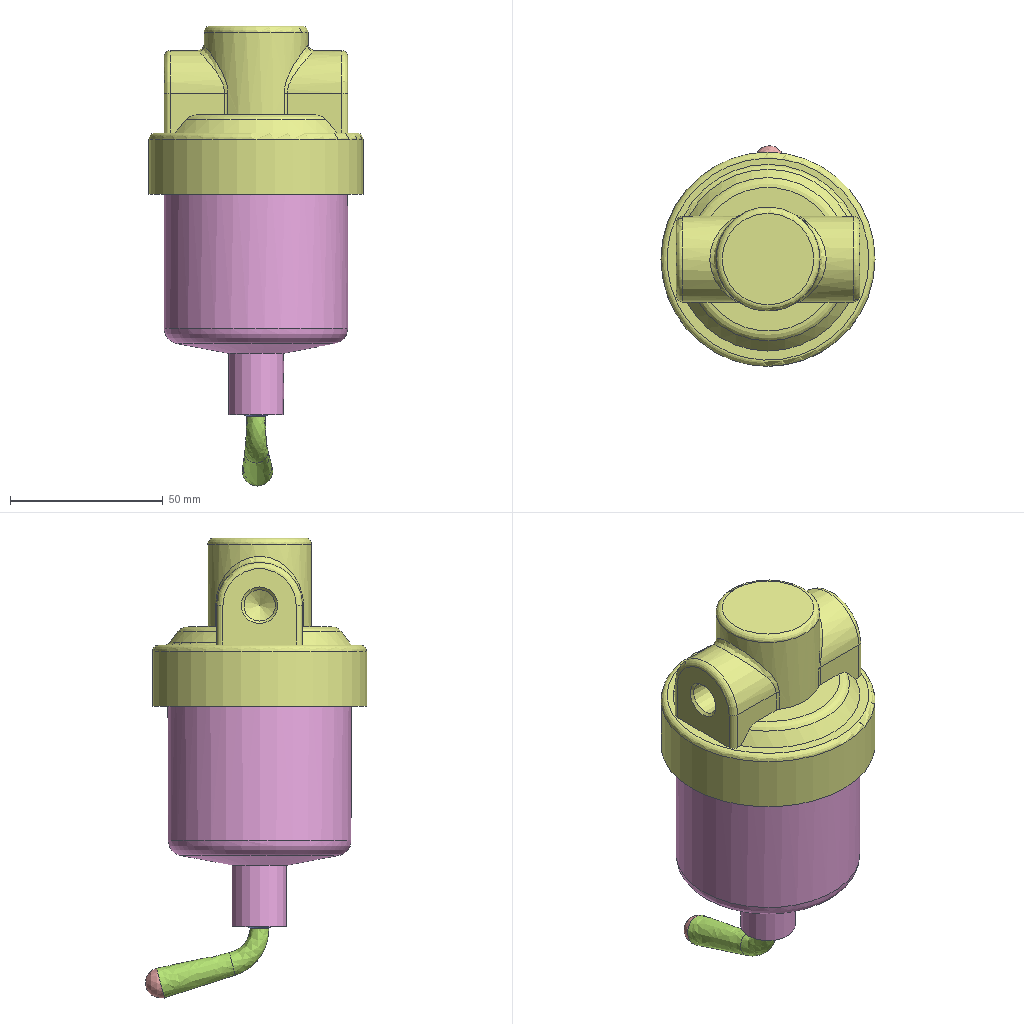Assembly | NX | 9 different items | 9 placed | box 70 x 72 x 150 mm
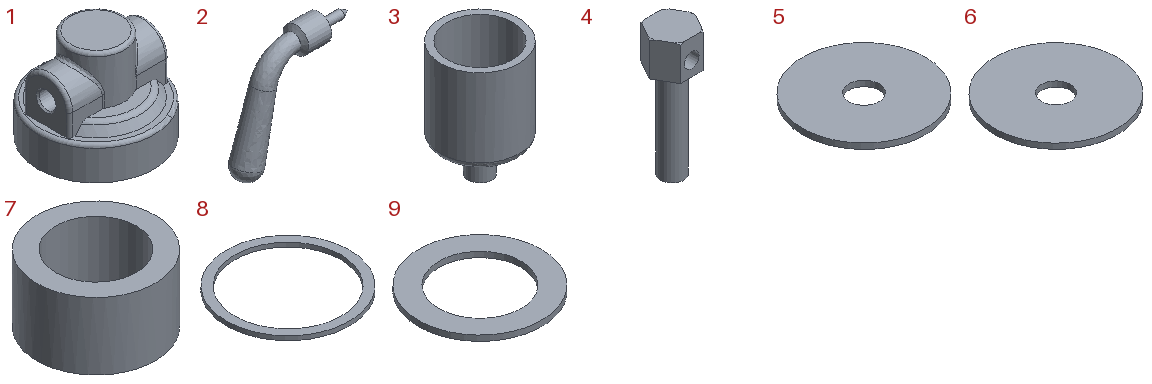Parts list (item | quantity | size | volume | features):
1 | x1 | 70 x 70 x 55 mm | 79994 mm3 | features CYLINDER 5, HOLE PACKAGE 5, SIMPLE HOLE 5, SYMBOLIC_THREAD 4, BLEND 3, DATUM_CSYS 2, BLOCK 1, SKETCH 1, SWP104 1
2 | x1 | 43.874 x 10 x 42.344 mm | 3412 mm3 | features SKETCH 4, DATUM_CSYS 3, DATUM_ON_PATH 2, SKIN 1, SPHERE 1, SWP104 1
3 | x1 | 60 x 60 x 88 mm | 68833 mm3 | features CYLINDER 3, BLEND 2, DATUM_CSYS 2, HOLE PACKAGE 2, SIMPLE HOLE 2, SYMBOLIC_THREAD 2, SKETCH 1, SWP104 1
4 | x1 | 18.475 x 16 x 52 mm | 4103 mm3 | features DATUM_CSYS 3, EXTRUDE 3, SKETCH 2, CHAMFER 1, CYLINDER 1, HOLE PACKAGE 1, SIMPLE HOLE 1, SYMBOLIC_THREAD 1
5 | x1 | 44 x 44 x 2 mm | 2851 mm3 | features CYLINDER 1, DATUM_CSYS 1, HOLE PACKAGE 1, SIMPLE HOLE 1
6 | x1 | 46 x 46 x 2 mm | 3134 mm3 | features CYLINDER 1, DATUM_CSYS 1, HOLE PACKAGE 1, SIMPLE HOLE 1
7 | x1 | 44.01 x 44.01 x 24.99 mm | 20351 mm3 | features CYLINDER 1, DATUM_CSYS 1, HOLE PACKAGE 1, SIMPLE HOLE 1
8 | x1 | 58 x 58 x 2 mm | 1357 mm3 | features CYLINDER 1, DATUM_CSYS 1, HOLE PACKAGE 1, SIMPLE HOLE 1
9 | x1 | 45 x 45 x 2 mm | 1767 mm3 | features CYLINDER 1, DATUM_CSYS 1, HOLE PACKAGE 1, SIMPLE HOLE 1